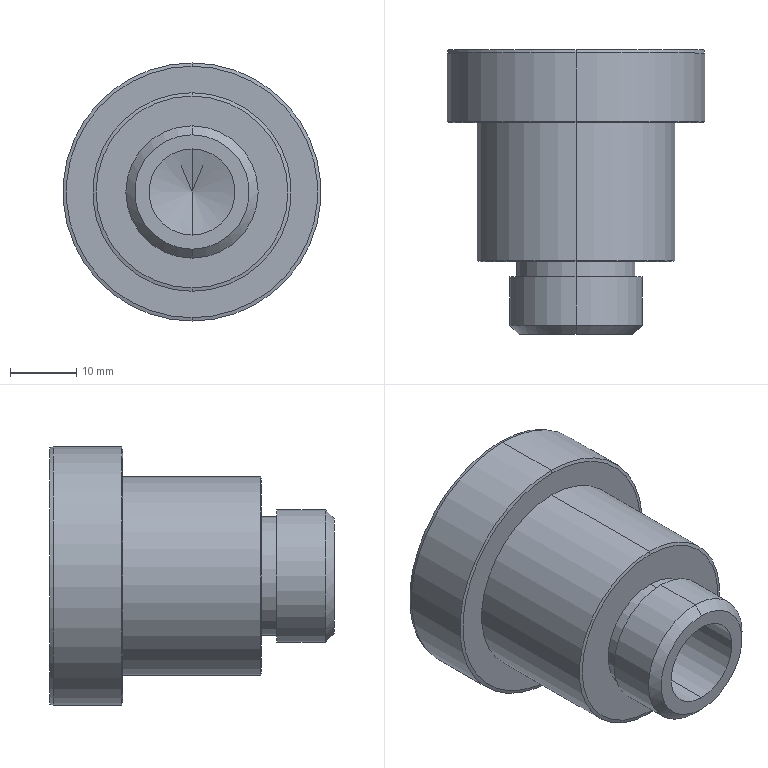Part | SolidWorks | features ICE 4, Chamfer 2, Extrusion 1, StudWizard 1 | 1 solid | 25 faces | box 39 x 43 x 39 mm | volume 27675 mm3 | cone 10 | cylinder 10 | plane 5 | commonest cylinder face diameters 13 x2 18 x2 20 x2 30 x2 39 x2
STEP:
#1=CARTESIAN_POINT('',(0.,6.645,-14.5));
#2=VERTEX_POINT('',#1);
#3=CARTESIAN_POINT('',(0.,6.645,14.5));
#4=VERTEX_POINT('',#3);
#5=CARTESIAN_POINT('',(0.,6.645,0.));
#6=DIRECTION('',(0.,-1.,0.));
#7=DIRECTION('',(0.,0.,1.));
#8=AXIS2_PLACEMENT_3D('',#5,#6,#7);
#9=CIRCLE('',#8,14.5);
#10=EDGE_CURVE('',#2,#4,#9,.T.);
#11=ORIENTED_EDGE('',*,*,#10,.F.);
#12=CARTESIAN_POINT('',(0.,6.779,-15.));
#13=VERTEX_POINT('',#12);
#14=CARTESIAN_POINT('',(0.,6.779,-15.));
#15=DIRECTION('',(0.,0.2588,-0.9659));
#16=VECTOR('',#15,1000.);
#17=LINE('',#14,#16);
#18=EDGE_CURVE('',#2,#13,#17,.T.);
#19=ORIENTED_EDGE('',*,*,#18,.T.);
#20=CARTESIAN_POINT('',(0.,6.779,15.));
#21=VERTEX_POINT('',#20);
#22=CARTESIAN_POINT('',(0.,6.779,0.));
#23=DIRECTION('',(0.,1.,0.));
#24=DIRECTION('',(0.,0.,1.));
#25=AXIS2_PLACEMENT_3D('',#22,#23,#24);
#26=CIRCLE('',#25,15.);
#27=EDGE_CURVE('',#21,#13,#26,.T.);
#28=ORIENTED_EDGE('',*,*,#27,.F.);
#29=CARTESIAN_POINT('',(0.,6.779,15.));
#30=DIRECTION('',(0.,0.2588,0.9659));
#31=VECTOR('',#30,1000.);
#32=LINE('',#29,#31);
#33=EDGE_CURVE('',#4,#21,#32,.T.);
#34=ORIENTED_EDGE('',*,*,#33,.F.);
#35=EDGE_LOOP('',(#11,#19,#28,#34));
#36=FACE_OUTER_BOUND('',#35,.T.);
#37=CARTESIAN_POINT('',(0.,6.779,0.));
#38=DIRECTION('',(0.,1.,0.));
#39=DIRECTION('',(0.,0.,1.));
#40=AXIS2_PLACEMENT_3D('',#37,#38,#39);
#41=CONICAL_SURFACE('',#40,15.,1.309);
#42=ADVANCED_FACE('',(#36),#41,.T.);
#43=CARTESIAN_POINT('',(0.,27.645,-19.));
#44=VERTEX_POINT('',#43);
#45=CARTESIAN_POINT('',(0.,27.645,19.));
#46=VERTEX_POINT('',#45);
#47=CARTESIAN_POINT('',(0.,27.645,0.));
#48=DIRECTION('',(0.,-1.,0.));
#49=DIRECTION('',(0.,0.,1.));
#50=AXIS2_PLACEMENT_3D('',#47,#48,#49);
#51=CIRCLE('',#50,19.);
#52=EDGE_CURVE('',#44,#46,#51,.T.);
#53=ORIENTED_EDGE('',*,*,#52,.F.);
#54=CARTESIAN_POINT('',(0.,27.779,-19.5));
#55=VERTEX_POINT('',#54);
#56=CARTESIAN_POINT('',(0.,27.779,-19.5));
#57=DIRECTION('',(0.,0.2588,-0.9659));
#58=VECTOR('',#57,1000.);
#59=LINE('',#56,#58);
#60=EDGE_CURVE('',#44,#55,#59,.T.);
#61=ORIENTED_EDGE('',*,*,#60,.T.);
#62=CARTESIAN_POINT('',(0.,27.779,19.5));
#63=VERTEX_POINT('',#62);
#64=CARTESIAN_POINT('',(0.,27.779,0.));
#65=DIRECTION('',(0.,1.,0.));
#66=DIRECTION('',(0.,0.,1.));
#67=AXIS2_PLACEMENT_3D('',#64,#65,#66);
#68=CIRCLE('',#67,19.5);
#69=EDGE_CURVE('',#63,#55,#68,.T.);
#70=ORIENTED_EDGE('',*,*,#69,.F.);
#71=CARTESIAN_POINT('',(0.,27.779,19.5));
#72=DIRECTION('',(0.,0.2588,0.9659));
#73=VECTOR('',#72,1000.);
#74=LINE('',#71,#73);
#75=EDGE_CURVE('',#46,#63,#74,.T.);
#76=ORIENTED_EDGE('',*,*,#75,.F.);
#77=EDGE_LOOP('',(#53,#61,#70,#76));
#78=FACE_OUTER_BOUND('',#77,.T.);
#79=CARTESIAN_POINT('',(0.,27.779,0.));
#80=DIRECTION('',(0.,1.,0.));
#81=DIRECTION('',(0.,0.,1.));
#82=AXIS2_PLACEMENT_3D('',#79,#80,#81);
#83=CONICAL_SURFACE('',#82,19.5,1.309);
#84=ADVANCED_FACE('',(#78),#83,.T.);
#85=CARTESIAN_POINT('',(0.,38.645,19.366));
#86=VERTEX_POINT('',#85);
#87=CARTESIAN_POINT('',(0.,38.645,-19.366));
#88=VERTEX_POINT('',#87);
#89=CARTESIAN_POINT('',(0.,38.645,0.));
#90=DIRECTION('',(0.,1.,0.));
#91=DIRECTION('',(0.,0.,1.));
#92=AXIS2_PLACEMENT_3D('',#89,#90,#91);
#93=CIRCLE('',#92,19.366);
#94=EDGE_CURVE('',#86,#88,#93,.T.);
#95=ORIENTED_EDGE('',*,*,#94,.F.);
#96=CARTESIAN_POINT('',(0.,38.145,19.5));
#97=VERTEX_POINT('',#96);
#98=CARTESIAN_POINT('',(0.,38.645,19.366));
#99=DIRECTION('',(0.,-0.9659,0.2588));
#100=VECTOR('',#99,1000.);
#101=LINE('',#98,#100);
#102=EDGE_CURVE('',#86,#97,#101,.T.);
#103=ORIENTED_EDGE('',*,*,#102,.T.);
#104=CARTESIAN_POINT('',(0.,38.145,-19.5));
#105=VERTEX_POINT('',#104);
#106=CARTESIAN_POINT('',(0.,38.145,0.));
#107=DIRECTION('',(0.,-1.,0.));
#108=DIRECTION('',(0.,0.,1.));
#109=AXIS2_PLACEMENT_3D('',#106,#107,#108);
#110=CIRCLE('',#109,19.5);
#111=EDGE_CURVE('',#105,#97,#110,.T.);
#112=ORIENTED_EDGE('',*,*,#111,.F.);
#113=CARTESIAN_POINT('',(0.,38.645,-19.366));
#114=DIRECTION('',(0.,-0.9659,-0.2588));
#115=VECTOR('',#114,1000.);
#116=LINE('',#113,#115);
#117=EDGE_CURVE('',#88,#105,#116,.T.);
#118=ORIENTED_EDGE('',*,*,#117,.F.);
#119=EDGE_LOOP('',(#95,#103,#112,#118));
#120=FACE_OUTER_BOUND('',#119,.T.);
#121=CARTESIAN_POINT('',(0.,38.645,0.));
#122=DIRECTION('',(0.,-1.,0.));
#123=DIRECTION('',(0.,0.,-1.));
#124=AXIS2_PLACEMENT_3D('',#121,#122,#123);
#125=CONICAL_SURFACE('',#124,19.366,0.2618);
#126=ADVANCED_FACE('',(#120),#125,.T.);
#127=CARTESIAN_POINT('',(0.,23.645,0.));
#128=VERTEX_POINT('',#127);
#129=CARTESIAN_POINT('',(0.,21.903,-6.5));
#130=VERTEX_POINT('',#129);
#131=CARTESIAN_POINT('',(0.,21.903,-6.5));
#132=DIRECTION('',(0.,-0.2588,-0.9659));
#133=VECTOR('',#132,1000.);
#134=LINE('',#131,#133);
#135=EDGE_CURVE('',#128,#130,#134,.T.);
#136=ORIENTED_EDGE('',*,*,#135,.F.);
#137=CARTESIAN_POINT('',(0.,21.903,6.5));
#138=VERTEX_POINT('',#137);
#139=CARTESIAN_POINT('',(0.,21.903,6.5));
#140=DIRECTION('',(0.,-0.2588,0.9659));
#141=VECTOR('',#140,1000.);
#142=LINE('',#139,#141);
#143=EDGE_CURVE('',#128,#138,#142,.T.);
#144=ORIENTED_EDGE('',*,*,#143,.T.);
#145=CARTESIAN_POINT('',(0.,21.903,0.));
#146=DIRECTION('',(0.,1.,0.));
#147=DIRECTION('',(0.,0.,-1.));
#148=AXIS2_PLACEMENT_3D('',#145,#146,#147);
#149=CIRCLE('',#148,6.5);
#150=EDGE_CURVE('',#130,#138,#149,.T.);
#151=ORIENTED_EDGE('',*,*,#150,.F.);
#152=EDGE_LOOP('',(#136,#144,#151));
#153=FACE_OUTER_BOUND('',#152,.T.);
#154=CARTESIAN_POINT('',(0.,21.903,0.));
#155=DIRECTION('',(0.,-1.,0.));
#156=DIRECTION('',(0.,0.,-1.));
#157=AXIS2_PLACEMENT_3D('',#154,#155,#156);
#158=CONICAL_SURFACE('',#157,6.5,1.309);
#159=ADVANCED_FACE('',(#153),#158,.F.);
#160=ORIENTED_EDGE('',*,*,#150,.T.);
#161=CARTESIAN_POINT('',(0.,-4.355,6.5));
#162=VERTEX_POINT('',#161);
#163=CARTESIAN_POINT('',(0.,23.645,6.5));
#164=DIRECTION('',(0.,-1.,0.));
#165=VECTOR('',#164,1000.);
#166=LINE('',#163,#165);
#167=EDGE_CURVE('',#138,#162,#166,.T.);
#168=ORIENTED_EDGE('',*,*,#167,.T.);
#169=CARTESIAN_POINT('',(0.,-4.355,-6.5));
#170=VERTEX_POINT('',#169);
#171=CARTESIAN_POINT('',(0.,-4.355,0.));
#172=DIRECTION('',(0.,-1.,0.));
#173=DIRECTION('',(0.,0.,-1.));
#174=AXIS2_PLACEMENT_3D('',#171,#172,#173);
#175=CIRCLE('',#174,6.5);
#176=EDGE_CURVE('',#162,#170,#175,.T.);
#177=ORIENTED_EDGE('',*,*,#176,.T.);
#178=CARTESIAN_POINT('',(0.,23.645,-6.5));
#179=DIRECTION('',(0.,-1.,0.));
#180=VECTOR('',#179,1000.);
#181=LINE('',#178,#180);
#182=EDGE_CURVE('',#130,#170,#181,.T.);
#183=ORIENTED_EDGE('',*,*,#182,.F.);
#184=EDGE_LOOP('',(#160,#168,#177,#183));
#185=FACE_OUTER_BOUND('',#184,.T.);
#186=CARTESIAN_POINT('',(0.,23.645,0.));
#187=DIRECTION('',(0.,-1.,0.));
#188=DIRECTION('',(0.,0.,-1.));
#189=AXIS2_PLACEMENT_3D('',#186,#187,#188);
#190=CYLINDRICAL_SURFACE('',#189,6.5);
#191=ADVANCED_FACE('',(#185),#190,.F.);
#192=CARTESIAN_POINT('',(0.,-4.355,8.647));
#193=VERTEX_POINT('',#192);
#194=CARTESIAN_POINT('',(0.,-4.355,-8.647));
#195=VERTEX_POINT('',#194);
#196=CARTESIAN_POINT('',(0.,-4.355,0.));
#197=DIRECTION('',(0.,1.,0.));
#198=DIRECTION('',(0.,0.,1.));
#199=AXIS2_PLACEMENT_3D('',#196,#197,#198);
#200=CIRCLE('',#199,8.647);
#201=EDGE_CURVE('',#193,#195,#200,.T.);
#202=ORIENTED_EDGE('',*,*,#201,.T.);
#203=CARTESIAN_POINT('',(0.,-3.002,-10.));
#204=VERTEX_POINT('',#203);
#205=CARTESIAN_POINT('',(0.,-4.355,-8.647));
#206=DIRECTION('',(0.,0.7071,-0.7071));
#207=VECTOR('',#206,1000.);
#208=LINE('',#205,#207);
#209=EDGE_CURVE('',#195,#204,#208,.T.);
#210=ORIENTED_EDGE('',*,*,#209,.T.);
#211=CARTESIAN_POINT('',(0.,-3.002,10.));
#212=VERTEX_POINT('',#211);
#213=CARTESIAN_POINT('',(0.,-3.002,0.));
#214=DIRECTION('',(0.,1.,0.));
#215=DIRECTION('',(0.,0.,1.));
#216=AXIS2_PLACEMENT_3D('',#213,#214,#215);
#217=CIRCLE('',#216,10.);
#218=EDGE_CURVE('',#212,#204,#217,.T.);
#219=ORIENTED_EDGE('',*,*,#218,.F.);
#220=CARTESIAN_POINT('',(0.,-4.355,8.647));
#221=DIRECTION('',(0.,0.7071,0.7071));
#222=VECTOR('',#221,1000.);
#223=LINE('',#220,#222);
#224=EDGE_CURVE('',#193,#212,#223,.T.);
#225=ORIENTED_EDGE('',*,*,#224,.F.);
#226=EDGE_LOOP('',(#202,#210,#219,#225));
#227=FACE_OUTER_BOUND('',#226,.T.);
#228=CARTESIAN_POINT('',(0.,-4.355,0.));
#229=DIRECTION('',(0.,1.,0.));
#230=DIRECTION('',(0.,0.,1.));
#231=AXIS2_PLACEMENT_3D('',#228,#229,#230);
#232=CONICAL_SURFACE('',#231,8.647,0.7854);
#233=ADVANCED_FACE('',(#227),#232,.T.);
#234=ORIENTED_EDGE('',*,*,#218,.T.);
#235=CARTESIAN_POINT('',(0.,4.355,-10.));
#236=VERTEX_POINT('',#235);
#237=CARTESIAN_POINT('',(0.,-4.355,-10.));
#238=DIRECTION('',(0.,1.,0.));
#239=VECTOR('',#238,1000.);
#240=LINE('',#237,#239);
#241=EDGE_CURVE('',#204,#236,#240,.T.);
#242=ORIENTED_EDGE('',*,*,#241,.T.);
#243=CARTESIAN_POINT('',(0.,4.355,10.));
#244=VERTEX_POINT('',#243);
#245=CARTESIAN_POINT('',(0.,4.355,0.));
#246=DIRECTION('',(0.,1.,0.));
#247=DIRECTION('',(0.,0.,1.));
#248=AXIS2_PLACEMENT_3D('',#245,#246,#247);
#249=CIRCLE('',#248,10.);
#250=EDGE_CURVE('',#244,#236,#249,.T.);
#251=ORIENTED_EDGE('',*,*,#250,.F.);
#252=CARTESIAN_POINT('',(0.,-4.355,10.));
#253=DIRECTION('',(0.,1.,0.));
#254=VECTOR('',#253,1000.);
#255=LINE('',#252,#254);
#256=EDGE_CURVE('',#212,#244,#255,.T.);
#257=ORIENTED_EDGE('',*,*,#256,.F.);
#258=EDGE_LOOP('',(#234,#242,#251,#257));
#259=FACE_OUTER_BOUND('',#258,.T.);
#260=CARTESIAN_POINT('',(0.,-4.355,0.));
#261=DIRECTION('',(0.,1.,0.));
#262=DIRECTION('',(0.,0.,1.));
#263=AXIS2_PLACEMENT_3D('',#260,#261,#262);
#264=CYLINDRICAL_SURFACE('',#263,10.);
#265=ADVANCED_FACE('',(#259),#264,.T.);
#266=ORIENTED_EDGE('',*,*,#111,.T.);
#267=CARTESIAN_POINT('',(0.,38.645,19.5));
#268=DIRECTION('',(0.,-1.,0.));
#269=VECTOR('',#268,1000.);
#270=LINE('',#267,#269);
#271=EDGE_CURVE('',#97,#63,#270,.T.);
#272=ORIENTED_EDGE('',*,*,#271,.T.);
#273=ORIENTED_EDGE('',*,*,#69,.T.);
#274=CARTESIAN_POINT('',(0.,38.645,-19.5));
#275=DIRECTION('',(0.,-1.,0.));
#276=VECTOR('',#275,1000.);
#277=LINE('',#274,#276);
#278=EDGE_CURVE('',#105,#55,#277,.T.);
#279=ORIENTED_EDGE('',*,*,#278,.F.);
#280=EDGE_LOOP('',(#266,#272,#273,#279));
#281=FACE_OUTER_BOUND('',#280,.T.);
#282=CARTESIAN_POINT('',(0.,38.645,0.));
#283=DIRECTION('',(0.,-1.,0.));
#284=DIRECTION('',(0.,0.,-1.));
#285=AXIS2_PLACEMENT_3D('',#282,#283,#284);
#286=CYLINDRICAL_SURFACE('',#285,19.5);
#287=ADVANCED_FACE('',(#281),#286,.T.);
#288=CARTESIAN_POINT('',(0.,27.645,15.));
#289=VERTEX_POINT('',#288);
#290=CARTESIAN_POINT('',(0.,27.645,-15.));
#291=VERTEX_POINT('',#290);
#292=CARTESIAN_POINT('',(0.,27.645,0.));
#293=DIRECTION('',(0.,1.,0.));
#294=DIRECTION('',(0.,0.,1.));
#295=AXIS2_PLACEMENT_3D('',#292,#293,#294);
#296=CIRCLE('',#295,15.);
#297=EDGE_CURVE('',#289,#291,#296,.T.);
#298=ORIENTED_EDGE('',*,*,#297,.F.);
#299=CARTESIAN_POINT('',(0.,27.645,15.));
#300=DIRECTION('',(0.,-1.,0.));
#301=VECTOR('',#300,1000.);
#302=LINE('',#299,#301);
#303=EDGE_CURVE('',#289,#21,#302,.T.);
#304=ORIENTED_EDGE('',*,*,#303,.T.);
#305=ORIENTED_EDGE('',*,*,#27,.T.);
#306=CARTESIAN_POINT('',(0.,27.645,-15.));
#307=DIRECTION('',(0.,-1.,0.));
#308=VECTOR('',#307,1000.);
#309=LINE('',#306,#308);
#310=EDGE_CURVE('',#291,#13,#309,.T.);
#311=ORIENTED_EDGE('',*,*,#310,.F.);
#312=EDGE_LOOP('',(#298,#304,#305,#311));
#313=FACE_OUTER_BOUND('',#312,.T.);
#314=CARTESIAN_POINT('',(0.,27.645,0.));
#315=DIRECTION('',(0.,-1.,0.));
#316=DIRECTION('',(0.,0.,-1.));
#317=AXIS2_PLACEMENT_3D('',#314,#315,#316);
#318=CYLINDRICAL_SURFACE('',#317,15.);
#319=ADVANCED_FACE('',(#313),#318,.T.);
#320=CARTESIAN_POINT('',(0.,6.645,9.));
#321=VERTEX_POINT('',#320);
#322=CARTESIAN_POINT('',(0.,6.645,-9.));
#323=VERTEX_POINT('',#322);
#324=CARTESIAN_POINT('',(0.,6.645,0.));
#325=DIRECTION('',(0.,1.,0.));
#326=DIRECTION('',(0.,0.,1.));
#327=AXIS2_PLACEMENT_3D('',#324,#325,#326);
#328=CIRCLE('',#327,9.);
#329=EDGE_CURVE('',#321,#323,#328,.T.);
#330=ORIENTED_EDGE('',*,*,#329,.F.);
#331=CARTESIAN_POINT('',(0.,4.355,9.));
#332=VERTEX_POINT('',#331);
#333=CARTESIAN_POINT('',(0.,6.645,9.));
#334=DIRECTION('',(0.,-1.,0.));
#335=VECTOR('',#334,1000.);
#336=LINE('',#333,#335);
#337=EDGE_CURVE('',#321,#332,#336,.T.);
#338=ORIENTED_EDGE('',*,*,#337,.T.);
#339=CARTESIAN_POINT('',(0.,4.355,-9.));
#340=VERTEX_POINT('',#339);
#341=CARTESIAN_POINT('',(0.,4.355,0.));
#342=DIRECTION('',(0.,1.,0.));
#343=DIRECTION('',(0.,0.,1.));
#344=AXIS2_PLACEMENT_3D('',#341,#342,#343);
#345=CIRCLE('',#344,9.);
#346=EDGE_CURVE('',#332,#340,#345,.T.);
#347=ORIENTED_EDGE('',*,*,#346,.T.);
#348=CARTESIAN_POINT('',(0.,6.645,-9.));
#349=DIRECTION('',(0.,-1.,0.));
#350=VECTOR('',#349,1000.);
#351=LINE('',#348,#350);
#352=EDGE_CURVE('',#323,#340,#351,.T.);
#353=ORIENTED_EDGE('',*,*,#352,.F.);
#354=EDGE_LOOP('',(#330,#338,#347,#353));
#355=FACE_OUTER_BOUND('',#354,.T.);
#356=CARTESIAN_POINT('',(0.,6.645,0.));
#357=DIRECTION('',(0.,-1.,0.));
#358=DIRECTION('',(0.,0.,-1.));
#359=AXIS2_PLACEMENT_3D('',#356,#357,#358);
#360=CYLINDRICAL_SURFACE('',#359,9.);
#361=ADVANCED_FACE('',(#355),#360,.T.);
#362=ORIENTED_EDGE('',*,*,#250,.T.);
#363=CARTESIAN_POINT('',(0.,4.355,0.));
#364=DIRECTION('',(0.,1.,0.));
#365=DIRECTION('',(0.,0.,1.));
#366=AXIS2_PLACEMENT_3D('',#363,#364,#365);
#367=CIRCLE('',#366,10.);
#368=EDGE_CURVE('',#236,#244,#367,.T.);
#369=ORIENTED_EDGE('',*,*,#368,.T.);
#370=EDGE_LOOP('',(#362,#369));
#371=FACE_OUTER_BOUND('',#370,.T.);
#372=CARTESIAN_POINT('',(0.,4.355,0.));
#373=DIRECTION('',(0.,1.,0.));
#374=DIRECTION('',(0.,0.,1.));
#375=AXIS2_PLACEMENT_3D('',#372,#373,#374);
#376=CIRCLE('',#375,9.);
#377=EDGE_CURVE('',#340,#332,#376,.T.);
#378=ORIENTED_EDGE('',*,*,#377,.F.);
#379=ORIENTED_EDGE('',*,*,#346,.F.);
#380=EDGE_LOOP('',(#378,#379));
#381=FACE_BOUND('',#380,.T.);
#382=CARTESIAN_POINT('',(0.,4.355,0.));
#383=DIRECTION('',(0.,1.,0.));
#384=DIRECTION('',(0.,0.,1.));
#385=AXIS2_PLACEMENT_3D('',#382,#383,#384);
#386=PLANE('',#385);
#387=ADVANCED_FACE('',(#371,#381),#386,.T.);
#388=ORIENTED_EDGE('',*,*,#337,.F.);
#389=CARTESIAN_POINT('',(0.,6.645,0.));
#390=DIRECTION('',(0.,1.,0.));
#391=DIRECTION('',(0.,0.,1.));
#392=AXIS2_PLACEMENT_3D('',#389,#390,#391);
#393=CIRCLE('',#392,9.);
#394=EDGE_CURVE('',#323,#321,#393,.T.);
#395=ORIENTED_EDGE('',*,*,#394,.F.);
#396=ORIENTED_EDGE('',*,*,#352,.T.);
#397=ORIENTED_EDGE('',*,*,#377,.T.);
#398=EDGE_LOOP('',(#388,#395,#396,#397));
#399=FACE_OUTER_BOUND('',#398,.T.);
#400=CARTESIAN_POINT('',(0.,6.645,0.));
#401=DIRECTION('',(0.,-1.,0.));
#402=DIRECTION('',(0.,0.,-1.));
#403=AXIS2_PLACEMENT_3D('',#400,#401,#402);
#404=CYLINDRICAL_SURFACE('',#403,9.);
#405=ADVANCED_FACE('',(#399),#404,.T.);
#406=ORIENTED_EDGE('',*,*,#303,.F.);
#407=CARTESIAN_POINT('',(0.,27.645,0.));
#408=DIRECTION('',(0.,1.,0.));
#409=DIRECTION('',(0.,0.,1.));
#410=AXIS2_PLACEMENT_3D('',#407,#408,#409);
#411=CIRCLE('',#410,15.);
#412=EDGE_CURVE('',#291,#289,#411,.T.);
#413=ORIENTED_EDGE('',*,*,#412,.F.);
#414=ORIENTED_EDGE('',*,*,#310,.T.);
#415=CARTESIAN_POINT('',(0.,6.779,0.));
#416=DIRECTION('',(0.,1.,0.));
#417=DIRECTION('',(0.,0.,1.));
#418=AXIS2_PLACEMENT_3D('',#415,#416,#417);
#419=CIRCLE('',#418,15.);
#420=EDGE_CURVE('',#13,#21,#419,.T.);
#421=ORIENTED_EDGE('',*,*,#420,.T.);
#422=EDGE_LOOP('',(#406,#413,#414,#421));
#423=FACE_OUTER_BOUND('',#422,.T.);
#424=CARTESIAN_POINT('',(0.,27.645,0.));
#425=DIRECTION('',(0.,-1.,0.));
#426=DIRECTION('',(0.,0.,-1.));
#427=AXIS2_PLACEMENT_3D('',#424,#425,#426);
#428=CYLINDRICAL_SURFACE('',#427,15.);
#429=ADVANCED_FACE('',(#423),#428,.T.);
#430=CARTESIAN_POINT('',(0.,6.645,0.));
#431=DIRECTION('',(0.,-1.,0.));
#432=DIRECTION('',(0.,0.,1.));
#433=AXIS2_PLACEMENT_3D('',#430,#431,#432);
#434=CIRCLE('',#433,14.5);
#435=EDGE_CURVE('',#4,#2,#434,.T.);
#436=ORIENTED_EDGE('',*,*,#435,.T.);
#437=ORIENTED_EDGE('',*,*,#10,.T.);
#438=EDGE_LOOP('',(#436,#437));
#439=FACE_OUTER_BOUND('',#438,.T.);
#440=ORIENTED_EDGE('',*,*,#394,.T.);
#441=ORIENTED_EDGE('',*,*,#329,.T.);
#442=EDGE_LOOP('',(#440,#441));
#443=FACE_BOUND('',#442,.T.);
#444=CARTESIAN_POINT('',(0.,6.645,0.));
#445=DIRECTION('',(0.,1.,0.));
#446=DIRECTION('',(0.,0.,1.));
#447=AXIS2_PLACEMENT_3D('',#444,#445,#446);
#448=PLANE('',#447);
#449=ADVANCED_FACE('',(#439,#443),#448,.F.);
#450=ORIENTED_EDGE('',*,*,#271,.F.);
#451=CARTESIAN_POINT('',(0.,38.145,0.));
#452=DIRECTION('',(0.,-1.,0.));
#453=DIRECTION('',(0.,0.,1.));
#454=AXIS2_PLACEMENT_3D('',#451,#452,#453);
#455=CIRCLE('',#454,19.5);
#456=EDGE_CURVE('',#97,#105,#455,.T.);
#457=ORIENTED_EDGE('',*,*,#456,.T.);
#458=ORIENTED_EDGE('',*,*,#278,.T.);
#459=CARTESIAN_POINT('',(0.,27.779,0.));
#460=DIRECTION('',(0.,1.,0.));
#461=DIRECTION('',(0.,0.,1.));
#462=AXIS2_PLACEMENT_3D('',#459,#460,#461);
#463=CIRCLE('',#462,19.5);
#464=EDGE_CURVE('',#55,#63,#463,.T.);
#465=ORIENTED_EDGE('',*,*,#464,.T.);
#466=EDGE_LOOP('',(#450,#457,#458,#465));
#467=FACE_OUTER_BOUND('',#466,.T.);
#468=CARTESIAN_POINT('',(0.,38.645,0.));
#469=DIRECTION('',(0.,-1.,0.));
#470=DIRECTION('',(0.,0.,-1.));
#471=AXIS2_PLACEMENT_3D('',#468,#469,#470);
#472=CYLINDRICAL_SURFACE('',#471,19.5);
#473=ADVANCED_FACE('',(#467),#472,.T.);
#474=CARTESIAN_POINT('',(0.,38.645,0.));
#475=DIRECTION('',(0.,1.,0.));
#476=DIRECTION('',(0.,0.,1.));
#477=AXIS2_PLACEMENT_3D('',#474,#475,#476);
#478=CIRCLE('',#477,19.366);
#479=EDGE_CURVE('',#88,#86,#478,.T.);
#480=ORIENTED_EDGE('',*,*,#479,.T.);
#481=ORIENTED_EDGE('',*,*,#94,.T.);
#482=EDGE_LOOP('',(#480,#481));
#483=FACE_OUTER_BOUND('',#482,.T.);
#484=CARTESIAN_POINT('',(0.,38.645,0.));
#485=DIRECTION('',(0.,1.,0.));
#486=DIRECTION('',(0.,0.,1.));
#487=AXIS2_PLACEMENT_3D('',#484,#485,#486);
#488=PLANE('',#487);
#489=ADVANCED_FACE('',(#483),#488,.T.);
#490=CARTESIAN_POINT('',(0.,27.645,0.));
#491=DIRECTION('',(0.,-1.,0.));
#492=DIRECTION('',(0.,0.,1.));
#493=AXIS2_PLACEMENT_3D('',#490,#491,#492);
#494=CIRCLE('',#493,19.);
#495=EDGE_CURVE('',#46,#44,#494,.T.);
#496=ORIENTED_EDGE('',*,*,#495,.T.);
#497=ORIENTED_EDGE('',*,*,#52,.T.);
#498=EDGE_LOOP('',(#496,#497));
#499=FACE_OUTER_BOUND('',#498,.T.);
#500=ORIENTED_EDGE('',*,*,#412,.T.);
#501=ORIENTED_EDGE('',*,*,#297,.T.);
#502=EDGE_LOOP('',(#500,#501));
#503=FACE_BOUND('',#502,.T.);
#504=CARTESIAN_POINT('',(0.,27.645,0.));
#505=DIRECTION('',(0.,1.,0.));
#506=DIRECTION('',(0.,0.,1.));
#507=AXIS2_PLACEMENT_3D('',#504,#505,#506);
#508=PLANE('',#507);
#509=ADVANCED_FACE('',(#499,#503),#508,.F.);
#510=ORIENTED_EDGE('',*,*,#241,.F.);
#511=CARTESIAN_POINT('',(0.,-3.002,0.));
#512=DIRECTION('',(0.,1.,0.));
#513=DIRECTION('',(0.,0.,1.));
#514=AXIS2_PLACEMENT_3D('',#511,#512,#513);
#515=CIRCLE('',#514,10.);
#516=EDGE_CURVE('',#204,#212,#515,.T.);
#517=ORIENTED_EDGE('',*,*,#516,.T.);
#518=ORIENTED_EDGE('',*,*,#256,.T.);
#519=ORIENTED_EDGE('',*,*,#368,.F.);
#520=EDGE_LOOP('',(#510,#517,#518,#519));
#521=FACE_OUTER_BOUND('',#520,.T.);
#522=CARTESIAN_POINT('',(0.,-4.355,0.));
#523=DIRECTION('',(0.,1.,0.));
#524=DIRECTION('',(0.,0.,1.));
#525=AXIS2_PLACEMENT_3D('',#522,#523,#524);
#526=CYLINDRICAL_SURFACE('',#525,10.);
#527=ADVANCED_FACE('',(#521),#526,.T.);
#528=ORIENTED_EDGE('',*,*,#209,.F.);
#529=CARTESIAN_POINT('',(0.,-4.355,0.));
#530=DIRECTION('',(0.,1.,0.));
#531=DIRECTION('',(0.,0.,1.));
#532=AXIS2_PLACEMENT_3D('',#529,#530,#531);
#533=CIRCLE('',#532,8.647);
#534=EDGE_CURVE('',#195,#193,#533,.T.);
#535=ORIENTED_EDGE('',*,*,#534,.T.);
#536=ORIENTED_EDGE('',*,*,#224,.T.);
#537=ORIENTED_EDGE('',*,*,#516,.F.);
#538=EDGE_LOOP('',(#528,#535,#536,#537));
#539=FACE_OUTER_BOUND('',#538,.T.);
#540=CARTESIAN_POINT('',(0.,-4.355,0.));
#541=DIRECTION('',(0.,1.,0.));
#542=DIRECTION('',(0.,0.,1.));
#543=AXIS2_PLACEMENT_3D('',#540,#541,#542);
#544=CONICAL_SURFACE('',#543,8.647,0.7854);
#545=ADVANCED_FACE('',(#539),#544,.T.);
#546=CARTESIAN_POINT('',(0.,-4.355,0.));
#547=DIRECTION('',(0.,-1.,0.));
#548=DIRECTION('',(0.,0.,-1.));
#549=AXIS2_PLACEMENT_3D('',#546,#547,#548);
#550=CIRCLE('',#549,6.5);
#551=EDGE_CURVE('',#170,#162,#550,.T.);
#552=ORIENTED_EDGE('',*,*,#551,.F.);
#553=ORIENTED_EDGE('',*,*,#176,.F.);
#554=EDGE_LOOP('',(#552,#553));
#555=FACE_BOUND('',#554,.T.);
#556=ORIENTED_EDGE('',*,*,#201,.F.);
#557=ORIENTED_EDGE('',*,*,#534,.F.);
#558=EDGE_LOOP('',(#556,#557));
#559=FACE_OUTER_BOUND('',#558,.T.);
#560=CARTESIAN_POINT('',(0.,-4.355,0.));
#561=DIRECTION('',(0.,1.,0.));
#562=DIRECTION('',(0.,0.,1.));
#563=AXIS2_PLACEMENT_3D('',#560,#561,#562);
#564=PLANE('',#563);
#565=ADVANCED_FACE('',(#555,#559),#564,.F.);
#566=ORIENTED_EDGE('',*,*,#167,.F.);
#567=CARTESIAN_POINT('',(0.,21.903,0.));
#568=DIRECTION('',(0.,1.,0.));
#569=DIRECTION('',(0.,0.,-1.));
#570=AXIS2_PLACEMENT_3D('',#567,#568,#569);
#571=CIRCLE('',#570,6.5);
#572=EDGE_CURVE('',#138,#130,#571,.T.);
#573=ORIENTED_EDGE('',*,*,#572,.T.);
#574=ORIENTED_EDGE('',*,*,#182,.T.);
#575=ORIENTED_EDGE('',*,*,#551,.T.);
#576=EDGE_LOOP('',(#566,#573,#574,#575));
#577=FACE_OUTER_BOUND('',#576,.T.);
#578=CARTESIAN_POINT('',(0.,23.645,0.));
#579=DIRECTION('',(0.,-1.,0.));
#580=DIRECTION('',(0.,0.,-1.));
#581=AXIS2_PLACEMENT_3D('',#578,#579,#580);
#582=CYLINDRICAL_SURFACE('',#581,6.5);
#583=ADVANCED_FACE('',(#577),#582,.F.);
#584=ORIENTED_EDGE('',*,*,#143,.F.);
#585=ORIENTED_EDGE('',*,*,#135,.T.);
#586=ORIENTED_EDGE('',*,*,#572,.F.);
#587=EDGE_LOOP('',(#584,#585,#586));
#588=FACE_OUTER_BOUND('',#587,.T.);
#589=CARTESIAN_POINT('',(0.,21.903,0.));
#590=DIRECTION('',(0.,-1.,0.));
#591=DIRECTION('',(0.,0.,-1.));
#592=AXIS2_PLACEMENT_3D('',#589,#590,#591);
#593=CONICAL_SURFACE('',#592,6.5,1.309);
#594=ADVANCED_FACE('',(#588),#593,.F.);
#595=ORIENTED_EDGE('',*,*,#102,.F.);
#596=ORIENTED_EDGE('',*,*,#479,.F.);
#597=ORIENTED_EDGE('',*,*,#117,.T.);
#598=ORIENTED_EDGE('',*,*,#456,.F.);
#599=EDGE_LOOP('',(#595,#596,#597,#598));
#600=FACE_OUTER_BOUND('',#599,.T.);
#601=CARTESIAN_POINT('',(0.,38.645,0.));
#602=DIRECTION('',(0.,-1.,0.));
#603=DIRECTION('',(0.,0.,-1.));
#604=AXIS2_PLACEMENT_3D('',#601,#602,#603);
#605=CONICAL_SURFACE('',#604,19.366,0.2618);
#606=ADVANCED_FACE('',(#600),#605,.T.);
#607=ORIENTED_EDGE('',*,*,#60,.F.);
#608=ORIENTED_EDGE('',*,*,#495,.F.);
#609=ORIENTED_EDGE('',*,*,#75,.T.);
#610=ORIENTED_EDGE('',*,*,#464,.F.);
#611=EDGE_LOOP('',(#607,#608,#609,#610));
#612=FACE_OUTER_BOUND('',#611,.T.);
#613=CARTESIAN_POINT('',(0.,27.779,0.));
#614=DIRECTION('',(0.,1.,0.));
#615=DIRECTION('',(0.,0.,1.));
#616=AXIS2_PLACEMENT_3D('',#613,#614,#615);
#617=CONICAL_SURFACE('',#616,19.5,1.309);
#618=ADVANCED_FACE('',(#612),#617,.T.);
#619=ORIENTED_EDGE('',*,*,#18,.F.);
#620=ORIENTED_EDGE('',*,*,#435,.F.);
#621=ORIENTED_EDGE('',*,*,#33,.T.);
#622=ORIENTED_EDGE('',*,*,#420,.F.);
#623=EDGE_LOOP('',(#619,#620,#621,#622));
#624=FACE_OUTER_BOUND('',#623,.T.);
#625=CARTESIAN_POINT('',(0.,6.779,0.));
#626=DIRECTION('',(0.,1.,0.));
#627=DIRECTION('',(0.,0.,1.));
#628=AXIS2_PLACEMENT_3D('',#625,#626,#627);
#629=CONICAL_SURFACE('',#628,15.,1.309);
#630=ADVANCED_FACE('',(#624),#629,.T.);
#631=CLOSED_SHELL('',(#42,#84,#126,#159,#191,#233,#265,#287,#319,#361,#387,#405,#429,#449,#473,#489,#509,#527,#545,#565,#583,#594,#606,#618,#630));
#632=MANIFOLD_SOLID_BREP('',#631);
#633=CARTESIAN_POINT('',(0.,0.,0.));
#634=DIRECTION('',(0.,0.,1.));
#635=DIRECTION('',(1.,0.,0.));
#636=AXIS2_PLACEMENT_3D('',#633,#634,#635);
#637=(LENGTH_UNIT()NAMED_UNIT(*)SI_UNIT(.MILLI.,.METRE.));
#638=UNCERTAINTY_MEASURE_WITH_UNIT(LENGTH_MEASURE(0.00001),#637,'','');
#639=(NAMED_UNIT(*)PLANE_ANGLE_UNIT()SI_UNIT($,.RADIAN.));
#640=(NAMED_UNIT(*)SI_UNIT($,.STERADIAN.)SOLID_ANGLE_UNIT());
#641=(GEOMETRIC_REPRESENTATION_CONTEXT(3)GLOBAL_UNCERTAINTY_ASSIGNED_CONTEXT((#638))GLOBAL_UNIT_ASSIGNED_CONTEXT((#637,#639,#640))REPRESENTATION_CONTEXT('',''));
#642=ADVANCED_BREP_SHAPE_REPRESENTATION('',(#632,#636),#641);